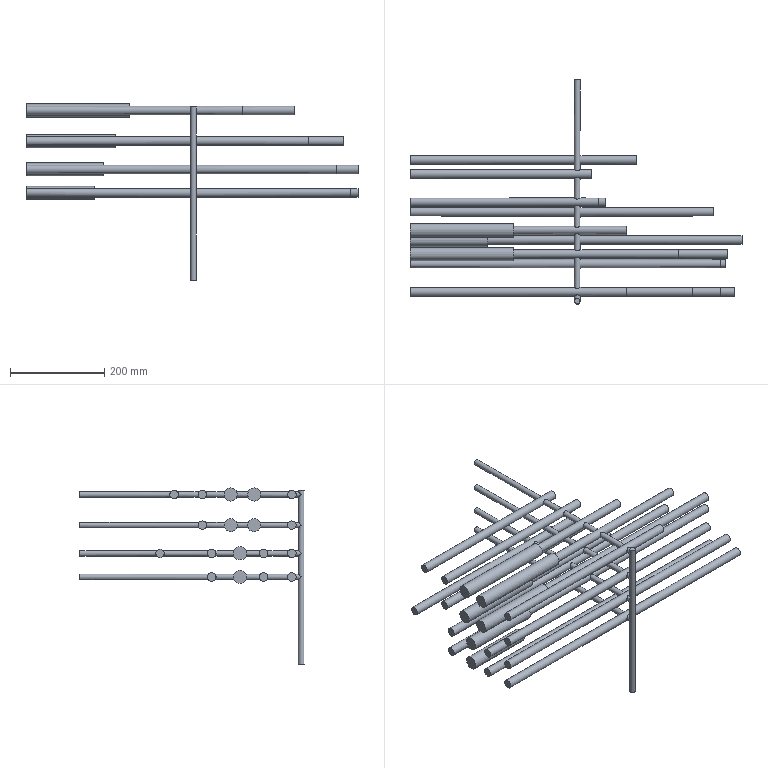Part | STEP file | solid 208 | 1 solid | 95 faces | box 705 x 476 x 374 mm | volume 3235310 mm3 | plane 48 | cylinder 47 | commonest cylinder face diameters 12 x23 18 x18 28 x6